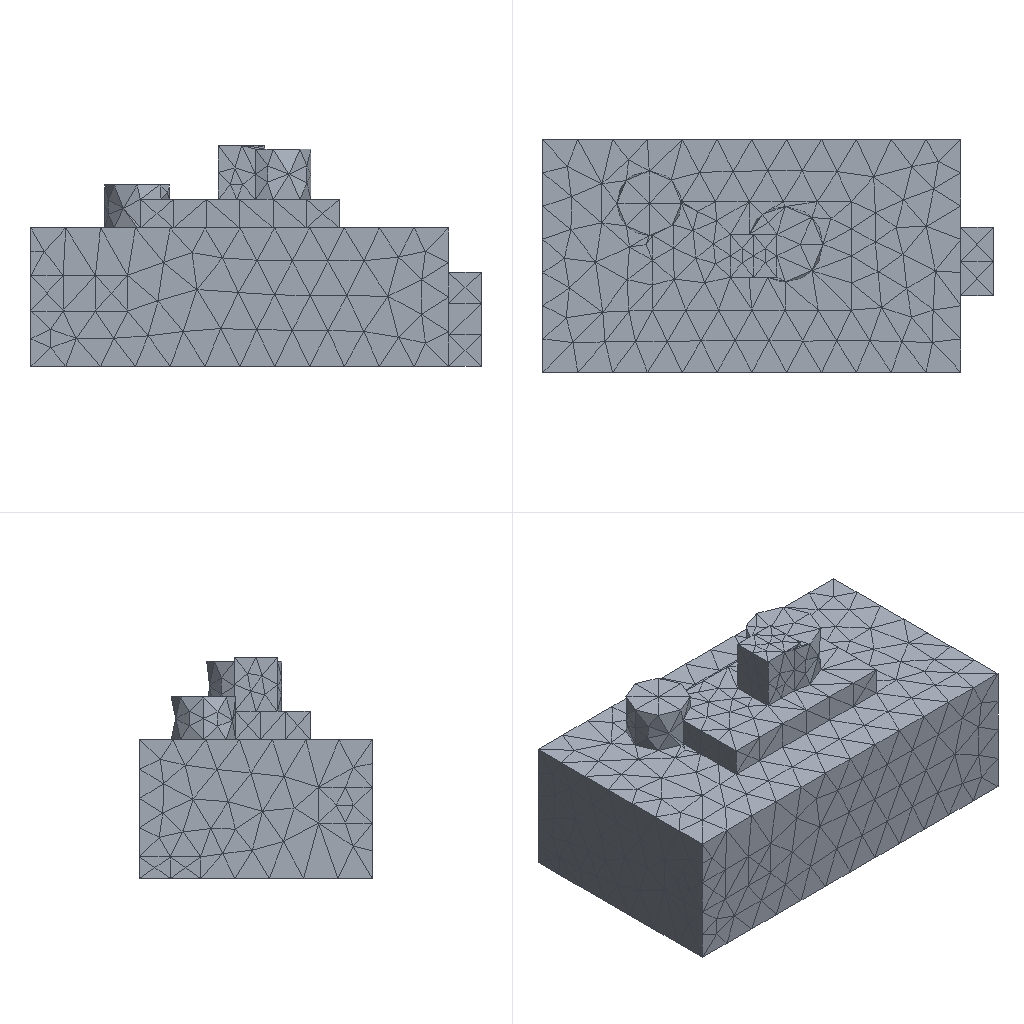Simulation study | ansys mapdl
Set-up summary:
category,name,step,type,value,unit,region
solver,ansys_mapdl
units,mm-N-s-tonne (MPa),,inferred,E=210000 density=
analysis,model,,static
mesh,nodes,,,6395
mesh,elements,,,3964
element_type,SOLID187,,,3964
material,mat 1,,E,210000
material,mat 1,,nu,0.3
load,,model,body load temp,,,all
load,,model,force,"1000 [dir=(0, 0, -1) n=449]",,node list
bc,,model,fixed,"[dofs=UX,UY,UZ n=5679]",,node list
Ansys APDL input file, long lists of numbers shortened:
/COM,ANSYS RELEASE 2026 R1           BUILD 26.1      UP20260202       09:08:28
/PREP7
/NOPR
/TITLE,2
ANTYPE, 0
*IF,_CDRDOFF,EQ,1,THEN     !if solid model was read in
_CDRDOFF=             !reset flag, numoffs already performed
*ELSE              !offset database for the following FE model
NUMOFF,NODE,     6395
NUMOFF,ELEM,     3964
NUMOFF,MAT ,        1
NUMOFF,TYPE,        1
*ENDIF
*SET,_RETURN ,  0.
*SET,_STATUS ,  0.
*SET,_UIQR   ,  449.
*SET,__FLOATPARAMETER__,  6395.
DOF,DELETE
ETBLOCK,        1,        1
(2i9,19a9)
        1      187        0        0        0        0        0        0        0        0        0        0        0        0        0        0        0        0        0        0        0
       -1
NBLOCK,6,SOLID,      6395,      6395
(3i9,6e21.13e3)
        1        0        0 7.0000000000000E+000 6.0000000000000E+000 6.1670000000000E+001
! (6394 more lines like these left out)
N,UNBL,LOC,       -1,
EBLOCK,19,SOLID,      3964,      3964
(19i10)
         1         1         1         1         0         0         0         0        10         0         1       197       195      2119      2123       196      2106      2107      2542
! (7927 more lines like these left out)
        -1
MPTEMP,UNBL, 1, 1,  0.    ,
MPDATA,UNBL, 1,EX  ,       1, 1,  210000.000    ,
MPTEMP,UNBL, 1, 1,  0.    ,
MPDATA,UNBL, 1,NUXY,       1, 1, 0.3    ,
MPTEMP,UNBL, 1, 1,  0.    ,
MPDATA,UNBL, 1,PRXY,       1, 1, 0.3    ,
EXTOPT,ATTR,      0,      0,      0
EXTOPT,ESIZE,  0,  0.
EXTOPT,ACLEAR,      0
TREF,  0.
IRLF,  0
BFUNIF,TEMP,_TINY
ACEL,  0.    ,  0.    ,  0.
OMEGA,  0.    ,  0.    ,  0.
DOMEGA,  0.    ,  0.    ,  0.
CGLOC,  0.    ,  0.    ,  0.
CGOMEGA,  0.    ,  0.    ,  0.
DCGOMG,  0.    ,  0.    ,  0.
KUSE,     0
TIME,  0.
ALPHAD,  0.
BETAD,  0.
DMPRAT,  0.
DMPSTR,  0.
CRPLIM, 0.1    ,   0
CRPLIM,  0.    ,   1
NCNV,     0, 1.000000000E+12,     0,  0.    ,  0.
NEQIT,     0
ERESX,DEFA
DBLOCK,      5679
(i9,a6,2(pg16.9))
      439  UX    0.00000000      0.00000000
! (5678 more lines like these left out)
       -1
FBLOCK,       449
(i9,a6,2(pg16.9))
        1  FZ   -2.22717149      0.00000000
! (448 more lines like these left out)
       -1
/GO
FINISH
Results summary:
result,analysis_type_db,,,static,unstated
result,n_sets,,,1,unstated
result,load_steps[0].set,load_step=1,,1,unstated
result,load_steps[0].substep,load_step=1,,1,unstated
result,load_steps[0].time,load_step=1,,1,unstated
result,load_steps[0].freq,load_step=1,,1,unstated
result,load_steps[0].max_usum,load_step=1,,0.0003927,unstated
result,load_steps[0].max_seqv,load_step=1,,4.578,unstated
result,load_steps[0].reaction_sum.FX,load_step=1,,2.46025e-12,unstated
result,load_steps[0].reaction_sum.FY,load_step=1,,-1.86797e-11,unstated
result,load_steps[0].reaction_sum.FZ,load_step=1,,1000,unstated
result,load_steps[0].reaction_sum.MX,load_step=1,,0,unstated
result,load_steps[0].reaction_sum.MY,load_step=1,,0,unstated
result,load_steps[0].reaction_sum.MZ,load_step=1,,0,unstated
result,convergence,,,results present for all listed sets,unstated